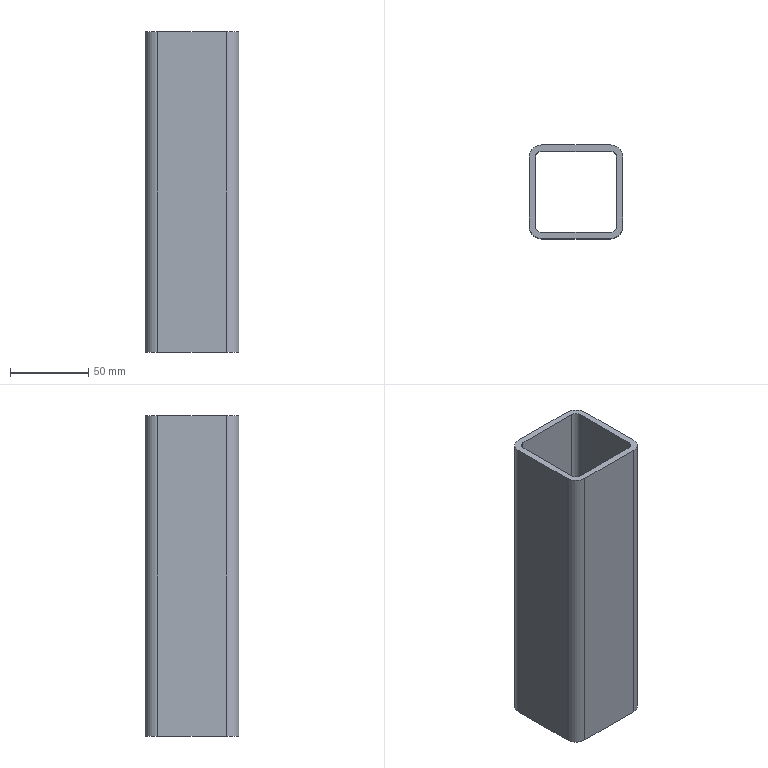Part | SolidWorks | features ICE 1, LibraryFeature 1 | 1 solid | 18 faces | box 60 x 60 x 205 mm | volume 175233 mm3 | plane 10 | cylinder 8 | commonest cylinder face diameters 8 x4 16 x4
STEP:
#1=CARTESIAN_POINT('',(22.,30.,0.));
#2=VERTEX_POINT('',#1);
#3=CARTESIAN_POINT('',(-22.,30.,0.));
#4=VERTEX_POINT('',#3);
#5=CARTESIAN_POINT('',(0.,30.,0.));
#6=DIRECTION('',(-1.,0.,0.));
#7=VECTOR('',#6,1000.);
#8=LINE('',#5,#7);
#9=EDGE_CURVE('',#2,#4,#8,.T.);
#10=ORIENTED_EDGE('',*,*,#9,.T.);
#11=CARTESIAN_POINT('',(-22.,30.,205.));
#12=VERTEX_POINT('',#11);
#13=CARTESIAN_POINT('',(-22.,30.,205.));
#14=DIRECTION('',(0.,0.,-1.));
#15=VECTOR('',#14,1000.);
#16=LINE('',#13,#15);
#17=EDGE_CURVE('',#12,#4,#16,.T.);
#18=ORIENTED_EDGE('',*,*,#17,.F.);
#19=CARTESIAN_POINT('',(22.,30.,205.));
#20=VERTEX_POINT('',#19);
#21=CARTESIAN_POINT('',(0.,30.,205.));
#22=DIRECTION('',(-1.,0.,0.));
#23=VECTOR('',#22,1000.);
#24=LINE('',#21,#23);
#25=EDGE_CURVE('',#20,#12,#24,.T.);
#26=ORIENTED_EDGE('',*,*,#25,.F.);
#27=CARTESIAN_POINT('',(22.,30.,205.));
#28=DIRECTION('',(0.,0.,-1.));
#29=VECTOR('',#28,1000.);
#30=LINE('',#27,#29);
#31=EDGE_CURVE('',#20,#2,#30,.T.);
#32=ORIENTED_EDGE('',*,*,#31,.T.);
#33=EDGE_LOOP('',(#10,#18,#26,#32));
#34=FACE_OUTER_BOUND('',#33,.T.);
#35=CARTESIAN_POINT('',(0.,30.,205.));
#36=DIRECTION('',(0.,-1.,0.));
#37=DIRECTION('',(0.,0.,-1.));
#38=AXIS2_PLACEMENT_3D('',#35,#36,#37);
#39=PLANE('',#38);
#40=ADVANCED_FACE('',(#34),#39,.F.);
#41=CARTESIAN_POINT('',(-30.,22.,0.));
#42=VERTEX_POINT('',#41);
#43=CARTESIAN_POINT('',(-22.,22.,0.));
#44=DIRECTION('',(0.,0.,1.));
#45=DIRECTION('',(1.,0.,0.));
#46=AXIS2_PLACEMENT_3D('',#43,#44,#45);
#47=CIRCLE('',#46,8.);
#48=EDGE_CURVE('',#4,#42,#47,.T.);
#49=ORIENTED_EDGE('',*,*,#48,.T.);
#50=CARTESIAN_POINT('',(-30.,22.,205.));
#51=VERTEX_POINT('',#50);
#52=CARTESIAN_POINT('',(-30.,22.,205.));
#53=DIRECTION('',(0.,0.,-1.));
#54=VECTOR('',#53,1000.);
#55=LINE('',#52,#54);
#56=EDGE_CURVE('',#51,#42,#55,.T.);
#57=ORIENTED_EDGE('',*,*,#56,.F.);
#58=CARTESIAN_POINT('',(-22.,22.,205.));
#59=DIRECTION('',(0.,0.,1.));
#60=DIRECTION('',(1.,0.,0.));
#61=AXIS2_PLACEMENT_3D('',#58,#59,#60);
#62=CIRCLE('',#61,8.);
#63=EDGE_CURVE('',#12,#51,#62,.T.);
#64=ORIENTED_EDGE('',*,*,#63,.F.);
#65=ORIENTED_EDGE('',*,*,#17,.T.);
#66=EDGE_LOOP('',(#49,#57,#64,#65));
#67=FACE_OUTER_BOUND('',#66,.T.);
#68=CARTESIAN_POINT('',(-22.,22.,205.));
#69=DIRECTION('',(0.,0.,-1.));
#70=DIRECTION('',(-1.,0.,0.));
#71=AXIS2_PLACEMENT_3D('',#68,#69,#70);
#72=CYLINDRICAL_SURFACE('',#71,8.);
#73=ADVANCED_FACE('',(#67),#72,.T.);
#74=CARTESIAN_POINT('',(-30.,-22.,0.));
#75=VERTEX_POINT('',#74);
#76=CARTESIAN_POINT('',(-30.,0.,0.));
#77=DIRECTION('',(0.,1.,0.));
#78=VECTOR('',#77,1000.);
#79=LINE('',#76,#78);
#80=EDGE_CURVE('',#75,#42,#79,.T.);
#81=ORIENTED_EDGE('',*,*,#80,.F.);
#82=CARTESIAN_POINT('',(-30.,-22.,205.));
#83=VERTEX_POINT('',#82);
#84=CARTESIAN_POINT('',(-30.,-22.,205.));
#85=DIRECTION('',(0.,0.,-1.));
#86=VECTOR('',#85,1000.);
#87=LINE('',#84,#86);
#88=EDGE_CURVE('',#83,#75,#87,.T.);
#89=ORIENTED_EDGE('',*,*,#88,.F.);
#90=CARTESIAN_POINT('',(-30.,0.,205.));
#91=DIRECTION('',(0.,1.,0.));
#92=VECTOR('',#91,1000.);
#93=LINE('',#90,#92);
#94=EDGE_CURVE('',#83,#51,#93,.T.);
#95=ORIENTED_EDGE('',*,*,#94,.T.);
#96=ORIENTED_EDGE('',*,*,#56,.T.);
#97=EDGE_LOOP('',(#81,#89,#95,#96));
#98=FACE_OUTER_BOUND('',#97,.T.);
#99=CARTESIAN_POINT('',(-30.,0.,205.));
#100=DIRECTION('',(-1.,0.,0.));
#101=DIRECTION('',(0.,0.,1.));
#102=AXIS2_PLACEMENT_3D('',#99,#100,#101);
#103=PLANE('',#102);
#104=ADVANCED_FACE('',(#98),#103,.T.);
#105=CARTESIAN_POINT('',(-22.,-30.,0.));
#106=VERTEX_POINT('',#105);
#107=CARTESIAN_POINT('',(-22.,-22.,0.));
#108=DIRECTION('',(0.,0.,1.));
#109=DIRECTION('',(1.,0.,0.));
#110=AXIS2_PLACEMENT_3D('',#107,#108,#109);
#111=CIRCLE('',#110,8.);
#112=EDGE_CURVE('',#75,#106,#111,.T.);
#113=ORIENTED_EDGE('',*,*,#112,.T.);
#114=CARTESIAN_POINT('',(-22.,-30.,205.));
#115=VERTEX_POINT('',#114);
#116=CARTESIAN_POINT('',(-22.,-30.,205.));
#117=DIRECTION('',(0.,0.,-1.));
#118=VECTOR('',#117,1000.);
#119=LINE('',#116,#118);
#120=EDGE_CURVE('',#115,#106,#119,.T.);
#121=ORIENTED_EDGE('',*,*,#120,.F.);
#122=CARTESIAN_POINT('',(-22.,-22.,205.));
#123=DIRECTION('',(0.,0.,1.));
#124=DIRECTION('',(1.,0.,0.));
#125=AXIS2_PLACEMENT_3D('',#122,#123,#124);
#126=CIRCLE('',#125,8.);
#127=EDGE_CURVE('',#83,#115,#126,.T.);
#128=ORIENTED_EDGE('',*,*,#127,.F.);
#129=ORIENTED_EDGE('',*,*,#88,.T.);
#130=EDGE_LOOP('',(#113,#121,#128,#129));
#131=FACE_OUTER_BOUND('',#130,.T.);
#132=CARTESIAN_POINT('',(-22.,-22.,205.));
#133=DIRECTION('',(0.,0.,-1.));
#134=DIRECTION('',(-1.,0.,0.));
#135=AXIS2_PLACEMENT_3D('',#132,#133,#134);
#136=CYLINDRICAL_SURFACE('',#135,8.);
#137=ADVANCED_FACE('',(#131),#136,.T.);
#138=CARTESIAN_POINT('',(22.,-30.,0.));
#139=VERTEX_POINT('',#138);
#140=CARTESIAN_POINT('',(0.,-30.,0.));
#141=DIRECTION('',(1.,0.,0.));
#142=VECTOR('',#141,1000.);
#143=LINE('',#140,#142);
#144=EDGE_CURVE('',#106,#139,#143,.T.);
#145=ORIENTED_EDGE('',*,*,#144,.T.);
#146=CARTESIAN_POINT('',(22.,-30.,205.));
#147=VERTEX_POINT('',#146);
#148=CARTESIAN_POINT('',(22.,-30.,205.));
#149=DIRECTION('',(0.,0.,-1.));
#150=VECTOR('',#149,1000.);
#151=LINE('',#148,#150);
#152=EDGE_CURVE('',#147,#139,#151,.T.);
#153=ORIENTED_EDGE('',*,*,#152,.F.);
#154=CARTESIAN_POINT('',(0.,-30.,205.));
#155=DIRECTION('',(1.,0.,0.));
#156=VECTOR('',#155,1000.);
#157=LINE('',#154,#156);
#158=EDGE_CURVE('',#115,#147,#157,.T.);
#159=ORIENTED_EDGE('',*,*,#158,.F.);
#160=ORIENTED_EDGE('',*,*,#120,.T.);
#161=EDGE_LOOP('',(#145,#153,#159,#160));
#162=FACE_OUTER_BOUND('',#161,.T.);
#163=CARTESIAN_POINT('',(0.,-30.,205.));
#164=DIRECTION('',(0.,1.,0.));
#165=DIRECTION('',(0.,0.,1.));
#166=AXIS2_PLACEMENT_3D('',#163,#164,#165);
#167=PLANE('',#166);
#168=ADVANCED_FACE('',(#162),#167,.F.);
#169=CARTESIAN_POINT('',(30.,-22.,0.));
#170=VERTEX_POINT('',#169);
#171=CARTESIAN_POINT('',(22.,-22.,0.));
#172=DIRECTION('',(0.,0.,1.));
#173=DIRECTION('',(1.,0.,0.));
#174=AXIS2_PLACEMENT_3D('',#171,#172,#173);
#175=CIRCLE('',#174,8.);
#176=EDGE_CURVE('',#139,#170,#175,.T.);
#177=ORIENTED_EDGE('',*,*,#176,.T.);
#178=CARTESIAN_POINT('',(30.,-22.,205.));
#179=VERTEX_POINT('',#178);
#180=CARTESIAN_POINT('',(30.,-22.,205.));
#181=DIRECTION('',(0.,0.,-1.));
#182=VECTOR('',#181,1000.);
#183=LINE('',#180,#182);
#184=EDGE_CURVE('',#179,#170,#183,.T.);
#185=ORIENTED_EDGE('',*,*,#184,.F.);
#186=CARTESIAN_POINT('',(22.,-22.,205.));
#187=DIRECTION('',(0.,0.,1.));
#188=DIRECTION('',(1.,0.,0.));
#189=AXIS2_PLACEMENT_3D('',#186,#187,#188);
#190=CIRCLE('',#189,8.);
#191=EDGE_CURVE('',#147,#179,#190,.T.);
#192=ORIENTED_EDGE('',*,*,#191,.F.);
#193=ORIENTED_EDGE('',*,*,#152,.T.);
#194=EDGE_LOOP('',(#177,#185,#192,#193));
#195=FACE_OUTER_BOUND('',#194,.T.);
#196=CARTESIAN_POINT('',(22.,-22.,205.));
#197=DIRECTION('',(0.,0.,-1.));
#198=DIRECTION('',(-1.,0.,0.));
#199=AXIS2_PLACEMENT_3D('',#196,#197,#198);
#200=CYLINDRICAL_SURFACE('',#199,8.);
#201=ADVANCED_FACE('',(#195),#200,.T.);
#202=CARTESIAN_POINT('',(30.,22.,0.));
#203=VERTEX_POINT('',#202);
#204=CARTESIAN_POINT('',(30.,0.,0.));
#205=DIRECTION('',(0.,-1.,0.));
#206=VECTOR('',#205,1000.);
#207=LINE('',#204,#206);
#208=EDGE_CURVE('',#203,#170,#207,.T.);
#209=ORIENTED_EDGE('',*,*,#208,.F.);
#210=CARTESIAN_POINT('',(30.,22.,205.));
#211=VERTEX_POINT('',#210);
#212=CARTESIAN_POINT('',(30.,22.,205.));
#213=DIRECTION('',(0.,0.,-1.));
#214=VECTOR('',#213,1000.);
#215=LINE('',#212,#214);
#216=EDGE_CURVE('',#211,#203,#215,.T.);
#217=ORIENTED_EDGE('',*,*,#216,.F.);
#218=CARTESIAN_POINT('',(30.,0.,205.));
#219=DIRECTION('',(0.,-1.,0.));
#220=VECTOR('',#219,1000.);
#221=LINE('',#218,#220);
#222=EDGE_CURVE('',#211,#179,#221,.T.);
#223=ORIENTED_EDGE('',*,*,#222,.T.);
#224=ORIENTED_EDGE('',*,*,#184,.T.);
#225=EDGE_LOOP('',(#209,#217,#223,#224));
#226=FACE_OUTER_BOUND('',#225,.T.);
#227=CARTESIAN_POINT('',(30.,0.,205.));
#228=DIRECTION('',(1.,0.,0.));
#229=DIRECTION('',(0.,0.,-1.));
#230=AXIS2_PLACEMENT_3D('',#227,#228,#229);
#231=PLANE('',#230);
#232=ADVANCED_FACE('',(#226),#231,.T.);
#233=CARTESIAN_POINT('',(-26.,-22.,0.));
#234=VERTEX_POINT('',#233);
#235=CARTESIAN_POINT('',(-22.,-26.,0.));
#236=VERTEX_POINT('',#235);
#237=CARTESIAN_POINT('',(-22.,-22.,0.));
#238=DIRECTION('',(0.,0.,1.));
#239=DIRECTION('',(1.,0.,0.));
#240=AXIS2_PLACEMENT_3D('',#237,#238,#239);
#241=CIRCLE('',#240,4.);
#242=EDGE_CURVE('',#234,#236,#241,.T.);
#243=ORIENTED_EDGE('',*,*,#242,.F.);
#244=CARTESIAN_POINT('',(-26.,-22.,205.));
#245=VERTEX_POINT('',#244);
#246=CARTESIAN_POINT('',(-26.,-22.,205.));
#247=DIRECTION('',(0.,0.,-1.));
#248=VECTOR('',#247,1000.);
#249=LINE('',#246,#248);
#250=EDGE_CURVE('',#245,#234,#249,.T.);
#251=ORIENTED_EDGE('',*,*,#250,.F.);
#252=CARTESIAN_POINT('',(-22.,-26.,205.));
#253=VERTEX_POINT('',#252);
#254=CARTESIAN_POINT('',(-22.,-22.,205.));
#255=DIRECTION('',(0.,0.,1.));
#256=DIRECTION('',(1.,0.,0.));
#257=AXIS2_PLACEMENT_3D('',#254,#255,#256);
#258=CIRCLE('',#257,4.);
#259=EDGE_CURVE('',#245,#253,#258,.T.);
#260=ORIENTED_EDGE('',*,*,#259,.T.);
#261=CARTESIAN_POINT('',(-22.,-26.,205.));
#262=DIRECTION('',(0.,0.,-1.));
#263=VECTOR('',#262,1000.);
#264=LINE('',#261,#263);
#265=EDGE_CURVE('',#253,#236,#264,.T.);
#266=ORIENTED_EDGE('',*,*,#265,.T.);
#267=EDGE_LOOP('',(#243,#251,#260,#266));
#268=FACE_OUTER_BOUND('',#267,.T.);
#269=CARTESIAN_POINT('',(-22.,-22.,205.));
#270=DIRECTION('',(0.,0.,-1.));
#271=DIRECTION('',(-1.,0.,0.));
#272=AXIS2_PLACEMENT_3D('',#269,#270,#271);
#273=CYLINDRICAL_SURFACE('',#272,4.);
#274=ADVANCED_FACE('',(#268),#273,.F.);
#275=CARTESIAN_POINT('',(-26.,22.,0.));
#276=VERTEX_POINT('',#275);
#277=CARTESIAN_POINT('',(-26.,0.,0.));
#278=DIRECTION('',(0.,1.,0.));
#279=VECTOR('',#278,1000.);
#280=LINE('',#277,#279);
#281=EDGE_CURVE('',#234,#276,#280,.T.);
#282=ORIENTED_EDGE('',*,*,#281,.T.);
#283=CARTESIAN_POINT('',(-26.,22.,205.));
#284=VERTEX_POINT('',#283);
#285=CARTESIAN_POINT('',(-26.,22.,205.));
#286=DIRECTION('',(0.,0.,-1.));
#287=VECTOR('',#286,1000.);
#288=LINE('',#285,#287);
#289=EDGE_CURVE('',#284,#276,#288,.T.);
#290=ORIENTED_EDGE('',*,*,#289,.F.);
#291=CARTESIAN_POINT('',(-26.,0.,205.));
#292=DIRECTION('',(0.,1.,0.));
#293=VECTOR('',#292,1000.);
#294=LINE('',#291,#293);
#295=EDGE_CURVE('',#245,#284,#294,.T.);
#296=ORIENTED_EDGE('',*,*,#295,.F.);
#297=ORIENTED_EDGE('',*,*,#250,.T.);
#298=EDGE_LOOP('',(#282,#290,#296,#297));
#299=FACE_OUTER_BOUND('',#298,.T.);
#300=CARTESIAN_POINT('',(-26.,0.,205.));
#301=DIRECTION('',(-1.,0.,0.));
#302=DIRECTION('',(0.,0.,1.));
#303=AXIS2_PLACEMENT_3D('',#300,#301,#302);
#304=PLANE('',#303);
#305=ADVANCED_FACE('',(#299),#304,.F.);
#306=CARTESIAN_POINT('',(-22.,26.,0.));
#307=VERTEX_POINT('',#306);
#308=CARTESIAN_POINT('',(-22.,22.,0.));
#309=DIRECTION('',(0.,0.,1.));
#310=DIRECTION('',(1.,0.,0.));
#311=AXIS2_PLACEMENT_3D('',#308,#309,#310);
#312=CIRCLE('',#311,4.);
#313=EDGE_CURVE('',#307,#276,#312,.T.);
#314=ORIENTED_EDGE('',*,*,#313,.F.);
#315=CARTESIAN_POINT('',(-22.,26.,205.));
#316=VERTEX_POINT('',#315);
#317=CARTESIAN_POINT('',(-22.,26.,205.));
#318=DIRECTION('',(0.,0.,-1.));
#319=VECTOR('',#318,1000.);
#320=LINE('',#317,#319);
#321=EDGE_CURVE('',#316,#307,#320,.T.);
#322=ORIENTED_EDGE('',*,*,#321,.F.);
#323=CARTESIAN_POINT('',(-22.,22.,205.));
#324=DIRECTION('',(0.,0.,1.));
#325=DIRECTION('',(1.,0.,0.));
#326=AXIS2_PLACEMENT_3D('',#323,#324,#325);
#327=CIRCLE('',#326,4.);
#328=EDGE_CURVE('',#316,#284,#327,.T.);
#329=ORIENTED_EDGE('',*,*,#328,.T.);
#330=ORIENTED_EDGE('',*,*,#289,.T.);
#331=EDGE_LOOP('',(#314,#322,#329,#330));
#332=FACE_OUTER_BOUND('',#331,.T.);
#333=CARTESIAN_POINT('',(-22.,22.,205.));
#334=DIRECTION('',(0.,0.,-1.));
#335=DIRECTION('',(-1.,0.,0.));
#336=AXIS2_PLACEMENT_3D('',#333,#334,#335);
#337=CYLINDRICAL_SURFACE('',#336,4.);
#338=ADVANCED_FACE('',(#332),#337,.F.);
#339=CARTESIAN_POINT('',(22.,26.,0.));
#340=VERTEX_POINT('',#339);
#341=CARTESIAN_POINT('',(0.,26.,0.));
#342=DIRECTION('',(-1.,0.,0.));
#343=VECTOR('',#342,1000.);
#344=LINE('',#341,#343);
#345=EDGE_CURVE('',#340,#307,#344,.T.);
#346=ORIENTED_EDGE('',*,*,#345,.F.);
#347=CARTESIAN_POINT('',(22.,26.,205.));
#348=VERTEX_POINT('',#347);
#349=CARTESIAN_POINT('',(22.,26.,205.));
#350=DIRECTION('',(0.,0.,-1.));
#351=VECTOR('',#350,1000.);
#352=LINE('',#349,#351);
#353=EDGE_CURVE('',#348,#340,#352,.T.);
#354=ORIENTED_EDGE('',*,*,#353,.F.);
#355=CARTESIAN_POINT('',(0.,26.,205.));
#356=DIRECTION('',(-1.,0.,0.));
#357=VECTOR('',#356,1000.);
#358=LINE('',#355,#357);
#359=EDGE_CURVE('',#348,#316,#358,.T.);
#360=ORIENTED_EDGE('',*,*,#359,.T.);
#361=ORIENTED_EDGE('',*,*,#321,.T.);
#362=EDGE_LOOP('',(#346,#354,#360,#361));
#363=FACE_OUTER_BOUND('',#362,.T.);
#364=CARTESIAN_POINT('',(0.,26.,205.));
#365=DIRECTION('',(0.,-1.,0.));
#366=DIRECTION('',(0.,0.,-1.));
#367=AXIS2_PLACEMENT_3D('',#364,#365,#366);
#368=PLANE('',#367);
#369=ADVANCED_FACE('',(#363),#368,.T.);
#370=CARTESIAN_POINT('',(26.,22.,0.));
#371=VERTEX_POINT('',#370);
#372=CARTESIAN_POINT('',(22.,22.,0.));
#373=DIRECTION('',(0.,0.,1.));
#374=DIRECTION('',(1.,0.,0.));
#375=AXIS2_PLACEMENT_3D('',#372,#373,#374);
#376=CIRCLE('',#375,4.);
#377=EDGE_CURVE('',#371,#340,#376,.T.);
#378=ORIENTED_EDGE('',*,*,#377,.F.);
#379=CARTESIAN_POINT('',(26.,22.,205.));
#380=VERTEX_POINT('',#379);
#381=CARTESIAN_POINT('',(26.,22.,205.));
#382=DIRECTION('',(0.,0.,-1.));
#383=VECTOR('',#382,1000.);
#384=LINE('',#381,#383);
#385=EDGE_CURVE('',#380,#371,#384,.T.);
#386=ORIENTED_EDGE('',*,*,#385,.F.);
#387=CARTESIAN_POINT('',(22.,22.,205.));
#388=DIRECTION('',(0.,0.,1.));
#389=DIRECTION('',(1.,0.,0.));
#390=AXIS2_PLACEMENT_3D('',#387,#388,#389);
#391=CIRCLE('',#390,4.);
#392=EDGE_CURVE('',#380,#348,#391,.T.);
#393=ORIENTED_EDGE('',*,*,#392,.T.);
#394=ORIENTED_EDGE('',*,*,#353,.T.);
#395=EDGE_LOOP('',(#378,#386,#393,#394));
#396=FACE_OUTER_BOUND('',#395,.T.);
#397=CARTESIAN_POINT('',(22.,22.,205.));
#398=DIRECTION('',(0.,0.,-1.));
#399=DIRECTION('',(-1.,0.,0.));
#400=AXIS2_PLACEMENT_3D('',#397,#398,#399);
#401=CYLINDRICAL_SURFACE('',#400,4.);
#402=ADVANCED_FACE('',(#396),#401,.F.);
#403=CARTESIAN_POINT('',(26.,-22.,0.));
#404=VERTEX_POINT('',#403);
#405=CARTESIAN_POINT('',(26.,0.,0.));
#406=DIRECTION('',(0.,-1.,0.));
#407=VECTOR('',#406,1000.);
#408=LINE('',#405,#407);
#409=EDGE_CURVE('',#371,#404,#408,.T.);
#410=ORIENTED_EDGE('',*,*,#409,.T.);
#411=CARTESIAN_POINT('',(26.,-22.,205.));
#412=VERTEX_POINT('',#411);
#413=CARTESIAN_POINT('',(26.,-22.,205.));
#414=DIRECTION('',(0.,0.,-1.));
#415=VECTOR('',#414,1000.);
#416=LINE('',#413,#415);
#417=EDGE_CURVE('',#412,#404,#416,.T.);
#418=ORIENTED_EDGE('',*,*,#417,.F.);
#419=CARTESIAN_POINT('',(26.,0.,205.));
#420=DIRECTION('',(0.,-1.,0.));
#421=VECTOR('',#420,1000.);
#422=LINE('',#419,#421);
#423=EDGE_CURVE('',#380,#412,#422,.T.);
#424=ORIENTED_EDGE('',*,*,#423,.F.);
#425=ORIENTED_EDGE('',*,*,#385,.T.);
#426=EDGE_LOOP('',(#410,#418,#424,#425));
#427=FACE_OUTER_BOUND('',#426,.T.);
#428=CARTESIAN_POINT('',(26.,0.,205.));
#429=DIRECTION('',(1.,0.,0.));
#430=DIRECTION('',(0.,0.,-1.));
#431=AXIS2_PLACEMENT_3D('',#428,#429,#430);
#432=PLANE('',#431);
#433=ADVANCED_FACE('',(#427),#432,.F.);
#434=CARTESIAN_POINT('',(22.,-26.,0.));
#435=VERTEX_POINT('',#434);
#436=CARTESIAN_POINT('',(22.,-22.,0.));
#437=DIRECTION('',(0.,0.,1.));
#438=DIRECTION('',(1.,0.,0.));
#439=AXIS2_PLACEMENT_3D('',#436,#437,#438);
#440=CIRCLE('',#439,4.);
#441=EDGE_CURVE('',#435,#404,#440,.T.);
#442=ORIENTED_EDGE('',*,*,#441,.F.);
#443=CARTESIAN_POINT('',(22.,-26.,205.));
#444=VERTEX_POINT('',#443);
#445=CARTESIAN_POINT('',(22.,-26.,205.));
#446=DIRECTION('',(0.,0.,-1.));
#447=VECTOR('',#446,1000.);
#448=LINE('',#445,#447);
#449=EDGE_CURVE('',#444,#435,#448,.T.);
#450=ORIENTED_EDGE('',*,*,#449,.F.);
#451=CARTESIAN_POINT('',(22.,-22.,205.));
#452=DIRECTION('',(0.,0.,1.));
#453=DIRECTION('',(1.,0.,0.));
#454=AXIS2_PLACEMENT_3D('',#451,#452,#453);
#455=CIRCLE('',#454,4.);
#456=EDGE_CURVE('',#444,#412,#455,.T.);
#457=ORIENTED_EDGE('',*,*,#456,.T.);
#458=ORIENTED_EDGE('',*,*,#417,.T.);
#459=EDGE_LOOP('',(#442,#450,#457,#458));
#460=FACE_OUTER_BOUND('',#459,.T.);
#461=CARTESIAN_POINT('',(22.,-22.,205.));
#462=DIRECTION('',(0.,0.,-1.));
#463=DIRECTION('',(-1.,0.,0.));
#464=AXIS2_PLACEMENT_3D('',#461,#462,#463);
#465=CYLINDRICAL_SURFACE('',#464,4.);
#466=ADVANCED_FACE('',(#460),#465,.F.);
#467=CARTESIAN_POINT('',(0.,-26.,0.));
#468=DIRECTION('',(1.,0.,0.));
#469=VECTOR('',#468,1000.);
#470=LINE('',#467,#469);
#471=EDGE_CURVE('',#236,#435,#470,.T.);
#472=ORIENTED_EDGE('',*,*,#471,.F.);
#473=ORIENTED_EDGE('',*,*,#265,.F.);
#474=CARTESIAN_POINT('',(0.,-26.,205.));
#475=DIRECTION('',(1.,0.,0.));
#476=VECTOR('',#475,1000.);
#477=LINE('',#474,#476);
#478=EDGE_CURVE('',#253,#444,#477,.T.);
#479=ORIENTED_EDGE('',*,*,#478,.T.);
#480=ORIENTED_EDGE('',*,*,#449,.T.);
#481=EDGE_LOOP('',(#472,#473,#479,#480));
#482=FACE_OUTER_BOUND('',#481,.T.);
#483=CARTESIAN_POINT('',(0.,-26.,205.));
#484=DIRECTION('',(0.,1.,0.));
#485=DIRECTION('',(0.,0.,1.));
#486=AXIS2_PLACEMENT_3D('',#483,#484,#485);
#487=PLANE('',#486);
#488=ADVANCED_FACE('',(#482),#487,.T.);
#489=CARTESIAN_POINT('',(22.,22.,0.));
#490=DIRECTION('',(0.,0.,1.));
#491=DIRECTION('',(1.,0.,0.));
#492=AXIS2_PLACEMENT_3D('',#489,#490,#491);
#493=CIRCLE('',#492,8.);
#494=EDGE_CURVE('',#203,#2,#493,.T.);
#495=ORIENTED_EDGE('',*,*,#494,.T.);
#496=ORIENTED_EDGE('',*,*,#31,.F.);
#497=CARTESIAN_POINT('',(22.,22.,205.));
#498=DIRECTION('',(0.,0.,1.));
#499=DIRECTION('',(1.,0.,0.));
#500=AXIS2_PLACEMENT_3D('',#497,#498,#499);
#501=CIRCLE('',#500,8.);
#502=EDGE_CURVE('',#211,#20,#501,.T.);
#503=ORIENTED_EDGE('',*,*,#502,.F.);
#504=ORIENTED_EDGE('',*,*,#216,.T.);
#505=EDGE_LOOP('',(#495,#496,#503,#504));
#506=FACE_OUTER_BOUND('',#505,.T.);
#507=CARTESIAN_POINT('',(22.,22.,205.));
#508=DIRECTION('',(0.,0.,-1.));
#509=DIRECTION('',(-1.,0.,0.));
#510=AXIS2_PLACEMENT_3D('',#507,#508,#509);
#511=CYLINDRICAL_SURFACE('',#510,8.);
#512=ADVANCED_FACE('',(#506),#511,.T.);
#513=ORIENTED_EDGE('',*,*,#259,.F.);
#514=ORIENTED_EDGE('',*,*,#295,.T.);
#515=ORIENTED_EDGE('',*,*,#328,.F.);
#516=ORIENTED_EDGE('',*,*,#359,.F.);
#517=ORIENTED_EDGE('',*,*,#392,.F.);
#518=ORIENTED_EDGE('',*,*,#423,.T.);
#519=ORIENTED_EDGE('',*,*,#456,.F.);
#520=ORIENTED_EDGE('',*,*,#478,.F.);
#521=EDGE_LOOP('',(#513,#514,#515,#516,#517,#518,#519,#520));
#522=FACE_BOUND('',#521,.T.);
#523=ORIENTED_EDGE('',*,*,#25,.T.);
#524=ORIENTED_EDGE('',*,*,#63,.T.);
#525=ORIENTED_EDGE('',*,*,#94,.F.);
#526=ORIENTED_EDGE('',*,*,#127,.T.);
#527=ORIENTED_EDGE('',*,*,#158,.T.);
#528=ORIENTED_EDGE('',*,*,#191,.T.);
#529=ORIENTED_EDGE('',*,*,#222,.F.);
#530=ORIENTED_EDGE('',*,*,#502,.T.);
#531=EDGE_LOOP('',(#523,#524,#525,#526,#527,#528,#529,#530));
#532=FACE_OUTER_BOUND('',#531,.T.);
#533=CARTESIAN_POINT('',(0.,0.,205.));
#534=DIRECTION('',(0.,0.,1.));
#535=DIRECTION('',(1.,0.,0.));
#536=AXIS2_PLACEMENT_3D('',#533,#534,#535);
#537=PLANE('',#536);
#538=ADVANCED_FACE('',(#522,#532),#537,.T.);
#539=ORIENTED_EDGE('',*,*,#242,.T.);
#540=ORIENTED_EDGE('',*,*,#471,.T.);
#541=ORIENTED_EDGE('',*,*,#441,.T.);
#542=ORIENTED_EDGE('',*,*,#409,.F.);
#543=ORIENTED_EDGE('',*,*,#377,.T.);
#544=ORIENTED_EDGE('',*,*,#345,.T.);
#545=ORIENTED_EDGE('',*,*,#313,.T.);
#546=ORIENTED_EDGE('',*,*,#281,.F.);
#547=EDGE_LOOP('',(#539,#540,#541,#542,#543,#544,#545,#546));
#548=FACE_BOUND('',#547,.T.);
#549=ORIENTED_EDGE('',*,*,#9,.F.);
#550=ORIENTED_EDGE('',*,*,#494,.F.);
#551=ORIENTED_EDGE('',*,*,#208,.T.);
#552=ORIENTED_EDGE('',*,*,#176,.F.);
#553=ORIENTED_EDGE('',*,*,#144,.F.);
#554=ORIENTED_EDGE('',*,*,#112,.F.);
#555=ORIENTED_EDGE('',*,*,#80,.T.);
#556=ORIENTED_EDGE('',*,*,#48,.F.);
#557=EDGE_LOOP('',(#549,#550,#551,#552,#553,#554,#555,#556));
#558=FACE_OUTER_BOUND('',#557,.T.);
#559=CARTESIAN_POINT('',(0.,0.,0.));
#560=DIRECTION('',(0.,0.,1.));
#561=DIRECTION('',(1.,0.,0.));
#562=AXIS2_PLACEMENT_3D('',#559,#560,#561);
#563=PLANE('',#562);
#564=ADVANCED_FACE('',(#548,#558),#563,.F.);
#565=CLOSED_SHELL('',(#40,#73,#104,#137,#168,#201,#232,#274,#305,#338,#369,#402,#433,#466,#488,#512,#538,#564));
#566=MANIFOLD_SOLID_BREP('',#565);
#567=CARTESIAN_POINT('',(0.,0.,0.));
#568=DIRECTION('',(0.,0.,1.));
#569=DIRECTION('',(1.,0.,0.));
#570=AXIS2_PLACEMENT_3D('',#567,#568,#569);
#571=(LENGTH_UNIT()NAMED_UNIT(*)SI_UNIT(.MILLI.,.METRE.));
#572=UNCERTAINTY_MEASURE_WITH_UNIT(LENGTH_MEASURE(0.00001),#571,'','');
#573=(NAMED_UNIT(*)PLANE_ANGLE_UNIT()SI_UNIT($,.RADIAN.));
#574=(NAMED_UNIT(*)SI_UNIT($,.STERADIAN.)SOLID_ANGLE_UNIT());
#575=(GEOMETRIC_REPRESENTATION_CONTEXT(3)GLOBAL_UNCERTAINTY_ASSIGNED_CONTEXT((#572))GLOBAL_UNIT_ASSIGNED_CONTEXT((#571,#573,#574))REPRESENTATION_CONTEXT('',''));
#576=ADVANCED_BREP_SHAPE_REPRESENTATION('',(#566,#570),#575);